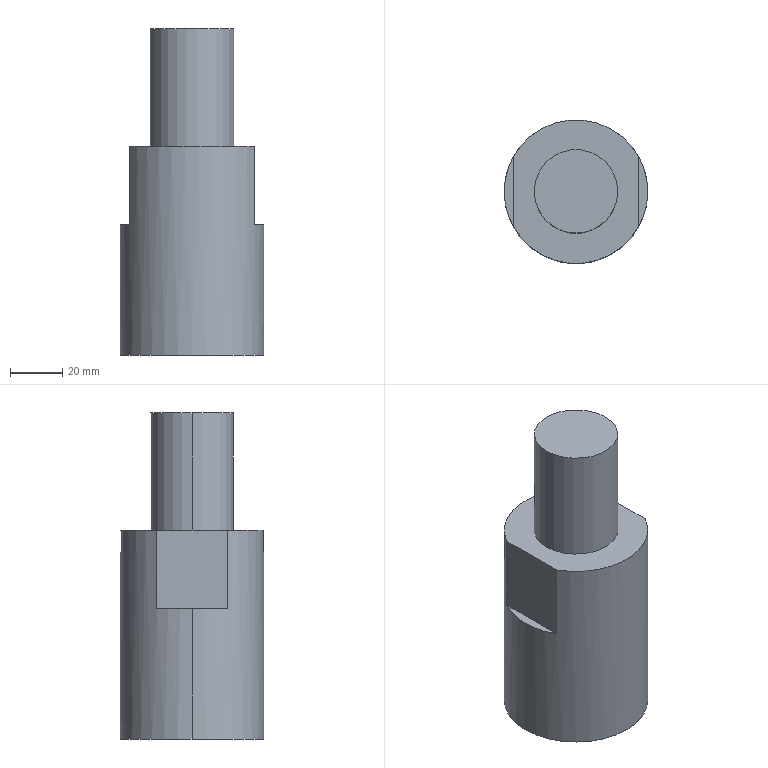Part | STEP file | 001-009-Riveting mechanism adapter joint | 1 solid | 15 faces | box 55 x 55 x 125 mm | volume 189803 mm3 | plane 7 | cylinder 6 | cone 2 | commonest cylinder face diameters 25 x2 32 x2 55 x2
STEP:
#1=CARTESIAN_POINT('',(0.,0.,0.));
#2=DIRECTION('',(0.,0.,1.));
#3=DIRECTION('',(1.,0.,0.));
#4=AXIS2_PLACEMENT_3D('',#1,#2,#3);
#5=CARTESIAN_POINT('',(-12.5,0.,64.));
#6=VERTEX_POINT('',#5);
#7=CARTESIAN_POINT('',(-12.5,0.,0.));
#8=VERTEX_POINT('',#7);
#9=CARTESIAN_POINT('',(-12.5,0.,0.));
#10=DIRECTION('',(0.,0.,-1.));
#11=VECTOR('',#10,1.);
#12=LINE('',#9,#11);
#13=CARTESIAN_POINT('',(0.,0.,0.));
#14=DIRECTION('',(0.,0.,-1.));
#15=DIRECTION('',(-1.,0.,0.));
#16=AXIS2_PLACEMENT_3D('',#13,#14,#15);
#17=CYLINDRICAL_SURFACE('',#16,12.5);
#18=CARTESIAN_POINT('',(6.283,0.));
#19=DIRECTION('',(0.,1.));
#20=VECTOR('',#19,1.);
#21=LINE('',#18,#20);
#22=(GEOMETRIC_REPRESENTATION_CONTEXT(2)PARAMETRIC_REPRESENTATION_CONTEXT()REPRESENTATION_CONTEXT('',''));
#23=DEFINITIONAL_REPRESENTATION('',(#21),#22);
#24=PCURVE('',#17,#23);
#25=CARTESIAN_POINT('',(0.,0.,0.));
#26=DIRECTION('',(0.,0.,-1.));
#27=DIRECTION('',(-1.,0.,0.));
#28=AXIS2_PLACEMENT_3D('',#25,#26,#27);
#29=CYLINDRICAL_SURFACE('',#28,12.5);
#30=CARTESIAN_POINT('',(0.,0.));
#31=DIRECTION('',(0.,1.));
#32=VECTOR('',#31,1.);
#33=LINE('',#30,#32);
#34=(GEOMETRIC_REPRESENTATION_CONTEXT(2)PARAMETRIC_REPRESENTATION_CONTEXT()REPRESENTATION_CONTEXT('',''));
#35=DEFINITIONAL_REPRESENTATION('',(#33),#34);
#36=PCURVE('',#29,#35);
#37=SURFACE_CURVE('',#12,(#24,#36),.PCURVE_S1.);
#38=EDGE_CURVE('',#6,#8,#37,.T.);
#39=ORIENTED_EDGE('',*,*,#38,.T.);
#40=CARTESIAN_POINT('',(12.5,0.,0.));
#41=VERTEX_POINT('',#40);
#42=CARTESIAN_POINT('',(0.,0.,0.));
#43=DIRECTION('',(0.,0.,-1.));
#44=DIRECTION('',(-1.,0.,0.));
#45=AXIS2_PLACEMENT_3D('',#42,#43,#44);
#46=CIRCLE('',#45,12.5);
#47=CARTESIAN_POINT('',(0.,0.));
#48=DIRECTION('',(1.,0.));
#49=VECTOR('',#48,1.);
#50=LINE('',#47,#49);
#51=(GEOMETRIC_REPRESENTATION_CONTEXT(2)PARAMETRIC_REPRESENTATION_CONTEXT()REPRESENTATION_CONTEXT('',''));
#52=DEFINITIONAL_REPRESENTATION('',(#50),#51);
#53=PCURVE('',#17,#52);
#54=CARTESIAN_POINT('',(0.,0.,0.));
#55=DIRECTION('',(0.,0.,1.));
#56=DIRECTION('',(1.,0.,0.));
#57=AXIS2_PLACEMENT_3D('',#54,#55,#56);
#58=PLANE('',#57);
#59=CARTESIAN_POINT('',(-12.5,0.));
#60=CARTESIAN_POINT('',(-12.5,21.651));
#61=CARTESIAN_POINT('',(6.25,10.825));
#62=CARTESIAN_POINT('',(25.,0.));
#63=CARTESIAN_POINT('',(6.25,-10.825));
#64=CARTESIAN_POINT('',(-12.5,-21.651));
#65=CARTESIAN_POINT('',(-12.5,0.));
#66=(BOUNDED_CURVE()B_SPLINE_CURVE(2,(#59,#60,#61,#62,#63,#64,#65),.UNSPECIFIED.,.T.,.F.)B_SPLINE_CURVE_WITH_KNOTS((1,2,2,2,2,1),(-2.094,0.,2.094,4.189,6.283,8.378),.UNSPECIFIED.)CURVE()GEOMETRIC_REPRESENTATION_ITEM()RATIONAL_B_SPLINE_CURVE((1.,0.5,1.,0.5,1.,0.5,1.))REPRESENTATION_ITEM(''));
#67=(GEOMETRIC_REPRESENTATION_CONTEXT(2)PARAMETRIC_REPRESENTATION_CONTEXT()REPRESENTATION_CONTEXT('',''));
#68=DEFINITIONAL_REPRESENTATION('',(#66),#67);
#69=PCURVE('',#58,#68);
#70=SURFACE_CURVE('',#46,(#53,#69),.PCURVE_S1.);
#71=EDGE_CURVE('',#41,#8,#70,.T.);
#72=ORIENTED_EDGE('',*,*,#71,.F.);
#73=CARTESIAN_POINT('',(12.5,0.,64.));
#74=VERTEX_POINT('',#73);
#75=CARTESIAN_POINT('',(12.5,0.,0.));
#76=DIRECTION('',(0.,0.,-1.));
#77=VECTOR('',#76,1.);
#78=LINE('',#75,#77);
#79=CARTESIAN_POINT('',(3.142,0.));
#80=DIRECTION('',(0.,1.));
#81=VECTOR('',#80,1.);
#82=LINE('',#79,#81);
#83=(GEOMETRIC_REPRESENTATION_CONTEXT(2)PARAMETRIC_REPRESENTATION_CONTEXT()REPRESENTATION_CONTEXT('',''));
#84=DEFINITIONAL_REPRESENTATION('',(#82),#83);
#85=PCURVE('',#17,#84);
#86=CARTESIAN_POINT('',(3.142,0.));
#87=DIRECTION('',(0.,1.));
#88=VECTOR('',#87,1.);
#89=LINE('',#86,#88);
#90=(GEOMETRIC_REPRESENTATION_CONTEXT(2)PARAMETRIC_REPRESENTATION_CONTEXT()REPRESENTATION_CONTEXT('',''));
#91=DEFINITIONAL_REPRESENTATION('',(#89),#90);
#92=PCURVE('',#29,#91);
#93=SURFACE_CURVE('',#78,(#85,#92),.PCURVE_S1.);
#94=EDGE_CURVE('',#74,#41,#93,.T.);
#95=ORIENTED_EDGE('',*,*,#94,.F.);
#96=CARTESIAN_POINT('',(0.,0.,64.));
#97=DIRECTION('',(0.,0.,-1.));
#98=DIRECTION('',(-1.,0.,0.));
#99=AXIS2_PLACEMENT_3D('',#96,#97,#98);
#100=CIRCLE('',#99,12.5);
#101=CARTESIAN_POINT('',(0.,-64.));
#102=DIRECTION('',(1.,0.));
#103=VECTOR('',#102,1.);
#104=LINE('',#101,#103);
#105=(GEOMETRIC_REPRESENTATION_CONTEXT(2)PARAMETRIC_REPRESENTATION_CONTEXT()REPRESENTATION_CONTEXT('',''));
#106=DEFINITIONAL_REPRESENTATION('',(#104),#105);
#107=PCURVE('',#17,#106);
#108=CARTESIAN_POINT('',(0.,0.,64.));
#109=DIRECTION('',(0.,0.,-1.));
#110=DIRECTION('',(-1.,0.,0.));
#111=AXIS2_PLACEMENT_3D('',#108,#109,#110);
#112=CONICAL_SURFACE('',#111,12.5,1.03);
#113=CARTESIAN_POINT('',(0.,0.));
#114=DIRECTION('',(1.,0.));
#115=VECTOR('',#114,1.);
#116=LINE('',#113,#115);
#117=(GEOMETRIC_REPRESENTATION_CONTEXT(2)PARAMETRIC_REPRESENTATION_CONTEXT()REPRESENTATION_CONTEXT('',''));
#118=DEFINITIONAL_REPRESENTATION('',(#116),#117);
#119=PCURVE('',#112,#118);
#120=SURFACE_CURVE('',#100,(#107,#119),.PCURVE_S1.);
#121=EDGE_CURVE('',#74,#6,#120,.T.);
#122=ORIENTED_EDGE('',*,*,#121,.T.);
#123=EDGE_LOOP('',(#39,#72,#95,#122));
#124=FACE_BOUND('',#123,.F.);
#125=ADVANCED_FACE('',(#124),#17,.F.);
#126=ORIENTED_EDGE('',*,*,#121,.F.);
#127=CARTESIAN_POINT('',(0.,0.,71.511));
#128=VERTEX_POINT('',#127);
#129=CARTESIAN_POINT('',(12.5,0.,64.));
#130=DIRECTION('',(0.8572,0.,-0.515));
#131=VECTOR('',#130,1.);
#132=LINE('',#129,#131);
#133=CARTESIAN_POINT('',(3.142,0.));
#134=DIRECTION('',(0.,1.));
#135=VECTOR('',#134,1.);
#136=LINE('',#133,#135);
#137=(GEOMETRIC_REPRESENTATION_CONTEXT(2)PARAMETRIC_REPRESENTATION_CONTEXT()REPRESENTATION_CONTEXT('',''));
#138=DEFINITIONAL_REPRESENTATION('',(#136),#137);
#139=PCURVE('',#112,#138);
#140=CARTESIAN_POINT('',(0.,0.,64.));
#141=DIRECTION('',(0.,0.,-1.));
#142=DIRECTION('',(-1.,0.,0.));
#143=AXIS2_PLACEMENT_3D('',#140,#141,#142);
#144=CONICAL_SURFACE('',#143,12.5,1.03);
#145=CARTESIAN_POINT('',(3.142,0.));
#146=DIRECTION('',(0.,1.));
#147=VECTOR('',#146,1.);
#148=LINE('',#145,#147);
#149=(GEOMETRIC_REPRESENTATION_CONTEXT(2)PARAMETRIC_REPRESENTATION_CONTEXT()REPRESENTATION_CONTEXT('',''));
#150=DEFINITIONAL_REPRESENTATION('',(#148),#149);
#151=PCURVE('',#144,#150);
#152=SURFACE_CURVE('',#132,(#139,#151),.PCURVE_S1.);
#153=EDGE_CURVE('',#128,#74,#152,.T.);
#154=ORIENTED_EDGE('',*,*,#153,.F.);
#155=CARTESIAN_POINT('',(-12.5,0.,64.));
#156=DIRECTION('',(-0.8572,0.,-0.515));
#157=VECTOR('',#156,1.);
#158=LINE('',#155,#157);
#159=CARTESIAN_POINT('',(6.283,0.));
#160=DIRECTION('',(0.,1.));
#161=VECTOR('',#160,1.);
#162=LINE('',#159,#161);
#163=(GEOMETRIC_REPRESENTATION_CONTEXT(2)PARAMETRIC_REPRESENTATION_CONTEXT()REPRESENTATION_CONTEXT('',''));
#164=DEFINITIONAL_REPRESENTATION('',(#162),#163);
#165=PCURVE('',#112,#164);
#166=CARTESIAN_POINT('',(0.,0.));
#167=DIRECTION('',(0.,1.));
#168=VECTOR('',#167,1.);
#169=LINE('',#166,#168);
#170=(GEOMETRIC_REPRESENTATION_CONTEXT(2)PARAMETRIC_REPRESENTATION_CONTEXT()REPRESENTATION_CONTEXT('',''));
#171=DEFINITIONAL_REPRESENTATION('',(#169),#170);
#172=PCURVE('',#144,#171);
#173=SURFACE_CURVE('',#158,(#165,#172),.PCURVE_S1.);
#174=EDGE_CURVE('',#128,#6,#173,.T.);
#175=ORIENTED_EDGE('',*,*,#174,.T.);
#176=EDGE_LOOP('',(#126,#154,#175));
#177=FACE_BOUND('',#176,.F.);
#178=ADVANCED_FACE('',(#177),#112,.F.);
#179=CARTESIAN_POINT('',(16.,0.,125.));
#180=VERTEX_POINT('',#179);
#181=CARTESIAN_POINT('',(-16.,0.,125.));
#182=VERTEX_POINT('',#181);
#183=CARTESIAN_POINT('',(0.,0.,125.));
#184=DIRECTION('',(0.,0.,1.));
#185=DIRECTION('',(1.,0.,0.));
#186=AXIS2_PLACEMENT_3D('',#183,#184,#185);
#187=CIRCLE('',#186,16.);
#188=CARTESIAN_POINT('',(0.,0.,125.));
#189=DIRECTION('',(0.,0.,-1.));
#190=DIRECTION('',(-1.,0.,0.));
#191=AXIS2_PLACEMENT_3D('',#188,#189,#190);
#192=CYLINDRICAL_SURFACE('',#191,16.);
#193=CARTESIAN_POINT('',(3.142,0.));
#194=DIRECTION('',(-1.,0.));
#195=VECTOR('',#194,1.);
#196=LINE('',#193,#195);
#197=(GEOMETRIC_REPRESENTATION_CONTEXT(2)PARAMETRIC_REPRESENTATION_CONTEXT()REPRESENTATION_CONTEXT('',''));
#198=DEFINITIONAL_REPRESENTATION('',(#196),#197);
#199=PCURVE('',#192,#198);
#200=CARTESIAN_POINT('',(0.,0.,125.));
#201=DIRECTION('',(0.,0.,1.));
#202=DIRECTION('',(1.,0.,0.));
#203=AXIS2_PLACEMENT_3D('',#200,#201,#202);
#204=PLANE('',#203);
#205=CARTESIAN_POINT('',(0.,0.));
#206=DIRECTION('',(1.,0.));
#207=AXIS2_PLACEMENT_2D('',#205,#206);
#208=CIRCLE('',#207,16.);
#209=(GEOMETRIC_REPRESENTATION_CONTEXT(2)PARAMETRIC_REPRESENTATION_CONTEXT()REPRESENTATION_CONTEXT('',''));
#210=DEFINITIONAL_REPRESENTATION('',(#208),#209);
#211=PCURVE('',#204,#210);
#212=SURFACE_CURVE('',#187,(#199,#211),.PCURVE_S1.);
#213=EDGE_CURVE('',#180,#182,#212,.T.);
#214=ORIENTED_EDGE('',*,*,#213,.F.);
#215=CARTESIAN_POINT('',(16.,0.,80.));
#216=VERTEX_POINT('',#215);
#217=CARTESIAN_POINT('',(16.,0.,125.));
#218=DIRECTION('',(0.,0.,-1.));
#219=VECTOR('',#218,1.);
#220=LINE('',#217,#219);
#221=CARTESIAN_POINT('',(3.142,0.));
#222=DIRECTION('',(0.,1.));
#223=VECTOR('',#222,1.);
#224=LINE('',#221,#223);
#225=(GEOMETRIC_REPRESENTATION_CONTEXT(2)PARAMETRIC_REPRESENTATION_CONTEXT()REPRESENTATION_CONTEXT('',''));
#226=DEFINITIONAL_REPRESENTATION('',(#224),#225);
#227=PCURVE('',#192,#226);
#228=CARTESIAN_POINT('',(0.,0.,125.));
#229=DIRECTION('',(0.,0.,-1.));
#230=DIRECTION('',(-1.,0.,0.));
#231=AXIS2_PLACEMENT_3D('',#228,#229,#230);
#232=CYLINDRICAL_SURFACE('',#231,16.);
#233=CARTESIAN_POINT('',(3.142,0.));
#234=DIRECTION('',(0.,1.));
#235=VECTOR('',#234,1.);
#236=LINE('',#233,#235);
#237=(GEOMETRIC_REPRESENTATION_CONTEXT(2)PARAMETRIC_REPRESENTATION_CONTEXT()REPRESENTATION_CONTEXT('',''));
#238=DEFINITIONAL_REPRESENTATION('',(#236),#237);
#239=PCURVE('',#232,#238);
#240=SURFACE_CURVE('',#220,(#227,#239),.PCURVE_S1.);
#241=EDGE_CURVE('',#180,#216,#240,.T.);
#242=ORIENTED_EDGE('',*,*,#241,.T.);
#243=CARTESIAN_POINT('',(-16.,0.,80.));
#244=VERTEX_POINT('',#243);
#245=CARTESIAN_POINT('',(0.,0.,80.));
#246=DIRECTION('',(0.,0.,1.));
#247=DIRECTION('',(1.,0.,0.));
#248=AXIS2_PLACEMENT_3D('',#245,#246,#247);
#249=CIRCLE('',#248,16.);
#250=CARTESIAN_POINT('',(3.142,45.));
#251=DIRECTION('',(-1.,0.));
#252=VECTOR('',#251,1.);
#253=LINE('',#250,#252);
#254=(GEOMETRIC_REPRESENTATION_CONTEXT(2)PARAMETRIC_REPRESENTATION_CONTEXT()REPRESENTATION_CONTEXT('',''));
#255=DEFINITIONAL_REPRESENTATION('',(#253),#254);
#256=PCURVE('',#192,#255);
#257=CARTESIAN_POINT('',(0.,0.,80.));
#258=DIRECTION('',(0.,0.,1.));
#259=DIRECTION('',(1.,0.,0.));
#260=AXIS2_PLACEMENT_3D('',#257,#258,#259);
#261=PLANE('',#260);
#262=CARTESIAN_POINT('',(0.,0.));
#263=DIRECTION('',(1.,0.));
#264=AXIS2_PLACEMENT_2D('',#262,#263);
#265=CIRCLE('',#264,16.);
#266=(GEOMETRIC_REPRESENTATION_CONTEXT(2)PARAMETRIC_REPRESENTATION_CONTEXT()REPRESENTATION_CONTEXT('',''));
#267=DEFINITIONAL_REPRESENTATION('',(#265),#266);
#268=PCURVE('',#261,#267);
#269=SURFACE_CURVE('',#249,(#256,#268),.PCURVE_S1.);
#270=EDGE_CURVE('',#216,#244,#269,.T.);
#271=ORIENTED_EDGE('',*,*,#270,.T.);
#272=CARTESIAN_POINT('',(-16.,0.,125.));
#273=DIRECTION('',(0.,0.,-1.));
#274=VECTOR('',#273,1.);
#275=LINE('',#272,#274);
#276=CARTESIAN_POINT('',(0.,0.));
#277=DIRECTION('',(0.,1.));
#278=VECTOR('',#277,1.);
#279=LINE('',#276,#278);
#280=(GEOMETRIC_REPRESENTATION_CONTEXT(2)PARAMETRIC_REPRESENTATION_CONTEXT()REPRESENTATION_CONTEXT('',''));
#281=DEFINITIONAL_REPRESENTATION('',(#279),#280);
#282=PCURVE('',#192,#281);
#283=CARTESIAN_POINT('',(6.283,0.));
#284=DIRECTION('',(0.,1.));
#285=VECTOR('',#284,1.);
#286=LINE('',#283,#285);
#287=(GEOMETRIC_REPRESENTATION_CONTEXT(2)PARAMETRIC_REPRESENTATION_CONTEXT()REPRESENTATION_CONTEXT('',''));
#288=DEFINITIONAL_REPRESENTATION('',(#286),#287);
#289=PCURVE('',#232,#288);
#290=SURFACE_CURVE('',#275,(#282,#289),.PCURVE_S1.);
#291=EDGE_CURVE('',#182,#244,#290,.T.);
#292=ORIENTED_EDGE('',*,*,#291,.F.);
#293=EDGE_LOOP('',(#214,#242,#271,#292));
#294=FACE_BOUND('',#293,.T.);
#295=ADVANCED_FACE('',(#294),#192,.T.);
#296=CARTESIAN_POINT('',(27.5,0.,50.));
#297=VERTEX_POINT('',#296);
#298=CARTESIAN_POINT('',(24.,13.426,50.));
#299=VERTEX_POINT('',#298);
#300=CARTESIAN_POINT('',(0.,0.,50.));
#301=DIRECTION('',(0.,0.,1.));
#302=DIRECTION('',(1.,0.,0.));
#303=AXIS2_PLACEMENT_3D('',#300,#301,#302);
#304=CIRCLE('',#303,27.5);
#305=CARTESIAN_POINT('',(0.,0.,80.));
#306=DIRECTION('',(0.,0.,-1.));
#307=DIRECTION('',(-1.,0.,0.));
#308=AXIS2_PLACEMENT_3D('',#305,#306,#307);
#309=CYLINDRICAL_SURFACE('',#308,27.5);
#310=CARTESIAN_POINT('',(3.142,30.));
#311=DIRECTION('',(-1.,0.));
#312=VECTOR('',#311,1.);
#313=LINE('',#310,#312);
#314=(GEOMETRIC_REPRESENTATION_CONTEXT(2)PARAMETRIC_REPRESENTATION_CONTEXT()REPRESENTATION_CONTEXT('',''));
#315=DEFINITIONAL_REPRESENTATION('',(#313),#314);
#316=PCURVE('',#309,#315);
#317=CARTESIAN_POINT('',(0.,0.,50.));
#318=DIRECTION('',(0.,0.,1.));
#319=DIRECTION('',(1.,0.,0.));
#320=AXIS2_PLACEMENT_3D('',#317,#318,#319);
#321=PLANE('',#320);
#322=CARTESIAN_POINT('',(0.,0.));
#323=DIRECTION('',(1.,0.));
#324=AXIS2_PLACEMENT_2D('',#322,#323);
#325=CIRCLE('',#324,27.5);
#326=(GEOMETRIC_REPRESENTATION_CONTEXT(2)PARAMETRIC_REPRESENTATION_CONTEXT()REPRESENTATION_CONTEXT('',''));
#327=DEFINITIONAL_REPRESENTATION('',(#325),#326);
#328=PCURVE('',#321,#327);
#329=SURFACE_CURVE('',#304,(#316,#328),.PCURVE_S1.);
#330=EDGE_CURVE('',#297,#299,#329,.T.);
#331=ORIENTED_EDGE('',*,*,#330,.F.);
#332=CARTESIAN_POINT('',(27.5,0.,0.));
#333=VERTEX_POINT('',#332);
#334=CARTESIAN_POINT('',(27.5,0.,80.));
#335=DIRECTION('',(0.,0.,-1.));
#336=VECTOR('',#335,1.);
#337=LINE('',#334,#336);
#338=CARTESIAN_POINT('',(3.142,0.));
#339=DIRECTION('',(0.,1.));
#340=VECTOR('',#339,1.);
#341=LINE('',#338,#340);
#342=(GEOMETRIC_REPRESENTATION_CONTEXT(2)PARAMETRIC_REPRESENTATION_CONTEXT()REPRESENTATION_CONTEXT('',''));
#343=DEFINITIONAL_REPRESENTATION('',(#341),#342);
#344=PCURVE('',#309,#343);
#345=CARTESIAN_POINT('',(0.,0.,80.));
#346=DIRECTION('',(0.,0.,-1.));
#347=DIRECTION('',(-1.,0.,0.));
#348=AXIS2_PLACEMENT_3D('',#345,#346,#347);
#349=CYLINDRICAL_SURFACE('',#348,27.5);
#350=CARTESIAN_POINT('',(3.142,0.));
#351=DIRECTION('',(0.,1.));
#352=VECTOR('',#351,1.);
#353=LINE('',#350,#352);
#354=(GEOMETRIC_REPRESENTATION_CONTEXT(2)PARAMETRIC_REPRESENTATION_CONTEXT()REPRESENTATION_CONTEXT('',''));
#355=DEFINITIONAL_REPRESENTATION('',(#353),#354);
#356=PCURVE('',#349,#355);
#357=SURFACE_CURVE('',#337,(#344,#356),.PCURVE_S1.);
#358=EDGE_CURVE('',#297,#333,#357,.T.);
#359=ORIENTED_EDGE('',*,*,#358,.T.);
#360=CARTESIAN_POINT('',(-27.5,0.,0.));
#361=VERTEX_POINT('',#360);
#362=CARTESIAN_POINT('',(0.,0.,0.));
#363=DIRECTION('',(0.,0.,1.));
#364=DIRECTION('',(1.,0.,0.));
#365=AXIS2_PLACEMENT_3D('',#362,#363,#364);
#366=CIRCLE('',#365,27.5);
#367=CARTESIAN_POINT('',(3.142,80.));
#368=DIRECTION('',(-1.,0.));
#369=VECTOR('',#368,1.);
#370=LINE('',#367,#369);
#371=(GEOMETRIC_REPRESENTATION_CONTEXT(2)PARAMETRIC_REPRESENTATION_CONTEXT()REPRESENTATION_CONTEXT('',''));
#372=DEFINITIONAL_REPRESENTATION('',(#370),#371);
#373=PCURVE('',#309,#372);
#374=CARTESIAN_POINT('',(0.,0.));
#375=DIRECTION('',(1.,0.));
#376=AXIS2_PLACEMENT_2D('',#374,#375);
#377=CIRCLE('',#376,27.5);
#378=(GEOMETRIC_REPRESENTATION_CONTEXT(2)PARAMETRIC_REPRESENTATION_CONTEXT()REPRESENTATION_CONTEXT('',''));
#379=DEFINITIONAL_REPRESENTATION('',(#377),#378);
#380=PCURVE('',#58,#379);
#381=SURFACE_CURVE('',#366,(#373,#380),.PCURVE_S1.);
#382=EDGE_CURVE('',#333,#361,#381,.T.);
#383=ORIENTED_EDGE('',*,*,#382,.T.);
#384=CARTESIAN_POINT('',(-27.5,0.,50.));
#385=VERTEX_POINT('',#384);
#386=CARTESIAN_POINT('',(-27.5,0.,80.));
#387=DIRECTION('',(0.,0.,-1.));
#388=VECTOR('',#387,1.);
#389=LINE('',#386,#388);
#390=CARTESIAN_POINT('',(0.,0.));
#391=DIRECTION('',(0.,1.));
#392=VECTOR('',#391,1.);
#393=LINE('',#390,#392);
#394=(GEOMETRIC_REPRESENTATION_CONTEXT(2)PARAMETRIC_REPRESENTATION_CONTEXT()REPRESENTATION_CONTEXT('',''));
#395=DEFINITIONAL_REPRESENTATION('',(#393),#394);
#396=PCURVE('',#309,#395);
#397=CARTESIAN_POINT('',(6.283,0.));
#398=DIRECTION('',(0.,1.));
#399=VECTOR('',#398,1.);
#400=LINE('',#397,#399);
#401=(GEOMETRIC_REPRESENTATION_CONTEXT(2)PARAMETRIC_REPRESENTATION_CONTEXT()REPRESENTATION_CONTEXT('',''));
#402=DEFINITIONAL_REPRESENTATION('',(#400),#401);
#403=PCURVE('',#349,#402);
#404=SURFACE_CURVE('',#389,(#396,#403),.PCURVE_S1.);
#405=EDGE_CURVE('',#385,#361,#404,.T.);
#406=ORIENTED_EDGE('',*,*,#405,.F.);
#407=CARTESIAN_POINT('',(-24.,13.426,50.));
#408=VERTEX_POINT('',#407);
#409=CARTESIAN_POINT('',(0.,0.,50.));
#410=DIRECTION('',(0.,0.,1.));
#411=DIRECTION('',(1.,0.,0.));
#412=AXIS2_PLACEMENT_3D('',#409,#410,#411);
#413=CIRCLE('',#412,27.5);
#414=CARTESIAN_POINT('',(3.142,30.));
#415=DIRECTION('',(-1.,0.));
#416=VECTOR('',#415,1.);
#417=LINE('',#414,#416);
#418=(GEOMETRIC_REPRESENTATION_CONTEXT(2)PARAMETRIC_REPRESENTATION_CONTEXT()REPRESENTATION_CONTEXT('',''));
#419=DEFINITIONAL_REPRESENTATION('',(#417),#418);
#420=PCURVE('',#309,#419);
#421=CARTESIAN_POINT('',(0.,0.,50.));
#422=DIRECTION('',(0.,0.,1.));
#423=DIRECTION('',(1.,0.,0.));
#424=AXIS2_PLACEMENT_3D('',#421,#422,#423);
#425=PLANE('',#424);
#426=CARTESIAN_POINT('',(0.,0.));
#427=DIRECTION('',(1.,0.));
#428=AXIS2_PLACEMENT_2D('',#426,#427);
#429=CIRCLE('',#428,27.5);
#430=(GEOMETRIC_REPRESENTATION_CONTEXT(2)PARAMETRIC_REPRESENTATION_CONTEXT()REPRESENTATION_CONTEXT('',''));
#431=DEFINITIONAL_REPRESENTATION('',(#429),#430);
#432=PCURVE('',#425,#431);
#433=SURFACE_CURVE('',#413,(#420,#432),.PCURVE_S1.);
#434=EDGE_CURVE('',#408,#385,#433,.T.);
#435=ORIENTED_EDGE('',*,*,#434,.F.);
#436=CARTESIAN_POINT('',(-24.,13.426,80.));
#437=VERTEX_POINT('',#436);
#438=CARTESIAN_POINT('',(-24.,13.426,80.));
#439=DIRECTION('',(0.,0.,-1.));
#440=VECTOR('',#439,1.);
#441=LINE('',#438,#440);
#442=CARTESIAN_POINT('',(0.51,0.));
#443=DIRECTION('',(0.,1.));
#444=VECTOR('',#443,1.);
#445=LINE('',#442,#444);
#446=(GEOMETRIC_REPRESENTATION_CONTEXT(2)PARAMETRIC_REPRESENTATION_CONTEXT()REPRESENTATION_CONTEXT('',''));
#447=DEFINITIONAL_REPRESENTATION('',(#445),#446);
#448=PCURVE('',#309,#447);
#449=CARTESIAN_POINT('',(-24.,-32.5,50.));
#450=DIRECTION('',(-1.,0.,0.));
#451=DIRECTION('',(0.,-1.,0.));
#452=AXIS2_PLACEMENT_3D('',#449,#450,#451);
#453=PLANE('',#452);
#454=CARTESIAN_POINT('',(-45.926,30.));
#455=DIRECTION('',(0.,-1.));
#456=VECTOR('',#455,1.);
#457=LINE('',#454,#456);
#458=(GEOMETRIC_REPRESENTATION_CONTEXT(2)PARAMETRIC_REPRESENTATION_CONTEXT()REPRESENTATION_CONTEXT('',''));
#459=DEFINITIONAL_REPRESENTATION('',(#457),#458);
#460=PCURVE('',#453,#459);
#461=SURFACE_CURVE('',#441,(#448,#460),.PCURVE_S1.);
#462=EDGE_CURVE('',#437,#408,#461,.T.);
#463=ORIENTED_EDGE('',*,*,#462,.F.);
#464=CARTESIAN_POINT('',(24.,13.426,80.));
#465=VERTEX_POINT('',#464);
#466=CARTESIAN_POINT('',(0.,0.,80.));
#467=DIRECTION('',(0.,0.,1.));
#468=DIRECTION('',(1.,0.,0.));
#469=AXIS2_PLACEMENT_3D('',#466,#467,#468);
#470=CIRCLE('',#469,27.5);
#471=CARTESIAN_POINT('',(3.142,0.));
#472=DIRECTION('',(-1.,0.));
#473=VECTOR('',#472,1.);
#474=LINE('',#471,#473);
#475=(GEOMETRIC_REPRESENTATION_CONTEXT(2)PARAMETRIC_REPRESENTATION_CONTEXT()REPRESENTATION_CONTEXT('',''));
#476=DEFINITIONAL_REPRESENTATION('',(#474),#475);
#477=PCURVE('',#309,#476);
#478=CARTESIAN_POINT('',(0.,0.));
#479=DIRECTION('',(1.,0.));
#480=AXIS2_PLACEMENT_2D('',#478,#479);
#481=CIRCLE('',#480,27.5);
#482=(GEOMETRIC_REPRESENTATION_CONTEXT(2)PARAMETRIC_REPRESENTATION_CONTEXT()REPRESENTATION_CONTEXT('',''));
#483=DEFINITIONAL_REPRESENTATION('',(#481),#482);
#484=PCURVE('',#261,#483);
#485=SURFACE_CURVE('',#470,(#477,#484),.PCURVE_S1.);
#486=EDGE_CURVE('',#465,#437,#485,.T.);
#487=ORIENTED_EDGE('',*,*,#486,.F.);
#488=CARTESIAN_POINT('',(24.,13.426,80.));
#489=DIRECTION('',(0.,0.,1.));
#490=VECTOR('',#489,1.);
#491=LINE('',#488,#490);
#492=CARTESIAN_POINT('',(2.632,0.));
#493=DIRECTION('',(0.,-1.));
#494=VECTOR('',#493,1.);
#495=LINE('',#492,#494);
#496=(GEOMETRIC_REPRESENTATION_CONTEXT(2)PARAMETRIC_REPRESENTATION_CONTEXT()REPRESENTATION_CONTEXT('',''));
#497=DEFINITIONAL_REPRESENTATION('',(#495),#496);
#498=PCURVE('',#309,#497);
#499=CARTESIAN_POINT('',(24.,-32.5,50.));
#500=DIRECTION('',(1.,0.,0.));
#501=DIRECTION('',(0.,1.,0.));
#502=AXIS2_PLACEMENT_3D('',#499,#500,#501);
#503=PLANE('',#502);
#504=CARTESIAN_POINT('',(45.926,30.));
#505=DIRECTION('',(0.,1.));
#506=VECTOR('',#505,1.);
#507=LINE('',#504,#506);
#508=(GEOMETRIC_REPRESENTATION_CONTEXT(2)PARAMETRIC_REPRESENTATION_CONTEXT()REPRESENTATION_CONTEXT('',''));
#509=DEFINITIONAL_REPRESENTATION('',(#507),#508);
#510=PCURVE('',#503,#509);
#511=SURFACE_CURVE('',#491,(#498,#510),.PCURVE_S1.);
#512=EDGE_CURVE('',#299,#465,#511,.T.);
#513=ORIENTED_EDGE('',*,*,#512,.F.);
#514=EDGE_LOOP('',(#331,#359,#383,#406,#435,#463,#487,#513));
#515=FACE_BOUND('',#514,.T.);
#516=ADVANCED_FACE('',(#515),#309,.T.);
#517=ORIENTED_EDGE('',*,*,#358,.F.);
#518=CARTESIAN_POINT('',(24.,-13.426,50.));
#519=VERTEX_POINT('',#518);
#520=CARTESIAN_POINT('',(0.,0.,50.));
#521=DIRECTION('',(0.,0.,1.));
#522=DIRECTION('',(1.,0.,0.));
#523=AXIS2_PLACEMENT_3D('',#520,#521,#522);
#524=CIRCLE('',#523,27.5);
#525=CARTESIAN_POINT('',(9.425,30.));
#526=DIRECTION('',(-1.,0.));
#527=VECTOR('',#526,1.);
#528=LINE('',#525,#527);
#529=(GEOMETRIC_REPRESENTATION_CONTEXT(2)PARAMETRIC_REPRESENTATION_CONTEXT()REPRESENTATION_CONTEXT('',''));
#530=DEFINITIONAL_REPRESENTATION('',(#528),#529);
#531=PCURVE('',#349,#530);
#532=CARTESIAN_POINT('',(0.,0.));
#533=DIRECTION('',(1.,0.));
#534=AXIS2_PLACEMENT_2D('',#532,#533);
#535=CIRCLE('',#534,27.5);
#536=(GEOMETRIC_REPRESENTATION_CONTEXT(2)PARAMETRIC_REPRESENTATION_CONTEXT()REPRESENTATION_CONTEXT('',''));
#537=DEFINITIONAL_REPRESENTATION('',(#535),#536);
#538=PCURVE('',#321,#537);
#539=SURFACE_CURVE('',#524,(#531,#538),.PCURVE_S1.);
#540=EDGE_CURVE('',#519,#297,#539,.T.);
#541=ORIENTED_EDGE('',*,*,#540,.F.);
#542=CARTESIAN_POINT('',(24.,-13.426,80.));
#543=VERTEX_POINT('',#542);
#544=CARTESIAN_POINT('',(24.,-13.426,80.));
#545=DIRECTION('',(0.,0.,-1.));
#546=VECTOR('',#545,1.);
#547=LINE('',#544,#546);
#548=CARTESIAN_POINT('',(3.652,0.));
#549=DIRECTION('',(0.,1.));
#550=VECTOR('',#549,1.);
#551=LINE('',#548,#550);
#552=(GEOMETRIC_REPRESENTATION_CONTEXT(2)PARAMETRIC_REPRESENTATION_CONTEXT()REPRESENTATION_CONTEXT('',''));
#553=DEFINITIONAL_REPRESENTATION('',(#551),#552);
#554=PCURVE('',#349,#553);
#555=CARTESIAN_POINT('',(19.074,30.));
#556=DIRECTION('',(0.,-1.));
#557=VECTOR('',#556,1.);
#558=LINE('',#555,#557);
#559=(GEOMETRIC_REPRESENTATION_CONTEXT(2)PARAMETRIC_REPRESENTATION_CONTEXT()REPRESENTATION_CONTEXT('',''));
#560=DEFINITIONAL_REPRESENTATION('',(#558),#559);
#561=PCURVE('',#503,#560);
#562=SURFACE_CURVE('',#547,(#554,#561),.PCURVE_S1.);
#563=EDGE_CURVE('',#543,#519,#562,.T.);
#564=ORIENTED_EDGE('',*,*,#563,.F.);
#565=CARTESIAN_POINT('',(-24.,-13.426,80.));
#566=VERTEX_POINT('',#565);
#567=CARTESIAN_POINT('',(0.,0.,80.));
#568=DIRECTION('',(0.,0.,1.));
#569=DIRECTION('',(1.,0.,0.));
#570=AXIS2_PLACEMENT_3D('',#567,#568,#569);
#571=CIRCLE('',#570,27.5);
#572=CARTESIAN_POINT('',(9.425,0.));
#573=DIRECTION('',(-1.,0.));
#574=VECTOR('',#573,1.);
#575=LINE('',#572,#574);
#576=(GEOMETRIC_REPRESENTATION_CONTEXT(2)PARAMETRIC_REPRESENTATION_CONTEXT()REPRESENTATION_CONTEXT('',''));
#577=DEFINITIONAL_REPRESENTATION('',(#575),#576);
#578=PCURVE('',#349,#577);
#579=CARTESIAN_POINT('',(0.,0.));
#580=DIRECTION('',(1.,0.));
#581=AXIS2_PLACEMENT_2D('',#579,#580);
#582=CIRCLE('',#581,27.5);
#583=(GEOMETRIC_REPRESENTATION_CONTEXT(2)PARAMETRIC_REPRESENTATION_CONTEXT()REPRESENTATION_CONTEXT('',''));
#584=DEFINITIONAL_REPRESENTATION('',(#582),#583);
#585=PCURVE('',#261,#584);
#586=SURFACE_CURVE('',#571,(#578,#585),.PCURVE_S1.);
#587=EDGE_CURVE('',#566,#543,#586,.T.);
#588=ORIENTED_EDGE('',*,*,#587,.F.);
#589=CARTESIAN_POINT('',(-24.,-13.426,50.));
#590=VERTEX_POINT('',#589);
#591=CARTESIAN_POINT('',(-24.,-13.426,80.));
#592=DIRECTION('',(0.,0.,1.));
#593=VECTOR('',#592,1.);
#594=LINE('',#591,#593);
#595=CARTESIAN_POINT('',(5.773,0.));
#596=DIRECTION('',(0.,-1.));
#597=VECTOR('',#596,1.);
#598=LINE('',#595,#597);
#599=(GEOMETRIC_REPRESENTATION_CONTEXT(2)PARAMETRIC_REPRESENTATION_CONTEXT()REPRESENTATION_CONTEXT('',''));
#600=DEFINITIONAL_REPRESENTATION('',(#598),#599);
#601=PCURVE('',#349,#600);
#602=CARTESIAN_POINT('',(-19.074,30.));
#603=DIRECTION('',(0.,1.));
#604=VECTOR('',#603,1.);
#605=LINE('',#602,#604);
#606=(GEOMETRIC_REPRESENTATION_CONTEXT(2)PARAMETRIC_REPRESENTATION_CONTEXT()REPRESENTATION_CONTEXT('',''));
#607=DEFINITIONAL_REPRESENTATION('',(#605),#606);
#608=PCURVE('',#453,#607);
#609=SURFACE_CURVE('',#594,(#601,#608),.PCURVE_S1.);
#610=EDGE_CURVE('',#590,#566,#609,.T.);
#611=ORIENTED_EDGE('',*,*,#610,.F.);
#612=CARTESIAN_POINT('',(0.,0.,50.));
#613=DIRECTION('',(0.,0.,1.));
#614=DIRECTION('',(1.,0.,0.));
#615=AXIS2_PLACEMENT_3D('',#612,#613,#614);
#616=CIRCLE('',#615,27.5);
#617=CARTESIAN_POINT('',(9.425,30.));
#618=DIRECTION('',(-1.,0.));
#619=VECTOR('',#618,1.);
#620=LINE('',#617,#619);
#621=(GEOMETRIC_REPRESENTATION_CONTEXT(2)PARAMETRIC_REPRESENTATION_CONTEXT()REPRESENTATION_CONTEXT('',''));
#622=DEFINITIONAL_REPRESENTATION('',(#620),#621);
#623=PCURVE('',#349,#622);
#624=CARTESIAN_POINT('',(0.,0.));
#625=DIRECTION('',(1.,0.));
#626=AXIS2_PLACEMENT_2D('',#624,#625);
#627=CIRCLE('',#626,27.5);
#628=(GEOMETRIC_REPRESENTATION_CONTEXT(2)PARAMETRIC_REPRESENTATION_CONTEXT()REPRESENTATION_CONTEXT('',''));
#629=DEFINITIONAL_REPRESENTATION('',(#627),#628);
#630=PCURVE('',#425,#629);
#631=SURFACE_CURVE('',#616,(#623,#630),.PCURVE_S1.);
#632=EDGE_CURVE('',#385,#590,#631,.T.);
#633=ORIENTED_EDGE('',*,*,#632,.F.);
#634=ORIENTED_EDGE('',*,*,#405,.T.);
#635=CARTESIAN_POINT('',(0.,0.,0.));
#636=DIRECTION('',(0.,0.,1.));
#637=DIRECTION('',(1.,0.,0.));
#638=AXIS2_PLACEMENT_3D('',#635,#636,#637);
#639=CIRCLE('',#638,27.5);
#640=CARTESIAN_POINT('',(9.425,80.));
#641=DIRECTION('',(-1.,0.));
#642=VECTOR('',#641,1.);
#643=LINE('',#640,#642);
#644=(GEOMETRIC_REPRESENTATION_CONTEXT(2)PARAMETRIC_REPRESENTATION_CONTEXT()REPRESENTATION_CONTEXT('',''));
#645=DEFINITIONAL_REPRESENTATION('',(#643),#644);
#646=PCURVE('',#349,#645);
#647=CARTESIAN_POINT('',(0.,0.));
#648=DIRECTION('',(1.,0.));
#649=AXIS2_PLACEMENT_2D('',#647,#648);
#650=CIRCLE('',#649,27.5);
#651=(GEOMETRIC_REPRESENTATION_CONTEXT(2)PARAMETRIC_REPRESENTATION_CONTEXT()REPRESENTATION_CONTEXT('',''));
#652=DEFINITIONAL_REPRESENTATION('',(#650),#651);
#653=PCURVE('',#58,#652);
#654=SURFACE_CURVE('',#639,(#646,#653),.PCURVE_S1.);
#655=EDGE_CURVE('',#361,#333,#654,.T.);
#656=ORIENTED_EDGE('',*,*,#655,.T.);
#657=EDGE_LOOP('',(#517,#541,#564,#588,#611,#633,#634,#656));
#658=FACE_BOUND('',#657,.T.);
#659=ADVANCED_FACE('',(#658),#349,.T.);
#660=CARTESIAN_POINT('',(0.,0.,80.));
#661=DIRECTION('',(0.,0.,1.));
#662=DIRECTION('',(1.,0.,0.));
#663=AXIS2_PLACEMENT_3D('',#660,#661,#662);
#664=CIRCLE('',#663,16.);
#665=CARTESIAN_POINT('',(0.,0.));
#666=DIRECTION('',(1.,0.));
#667=AXIS2_PLACEMENT_2D('',#665,#666);
#668=CIRCLE('',#667,16.);
#669=(GEOMETRIC_REPRESENTATION_CONTEXT(2)PARAMETRIC_REPRESENTATION_CONTEXT()REPRESENTATION_CONTEXT('',''));
#670=DEFINITIONAL_REPRESENTATION('',(#668),#669);
#671=PCURVE('',#261,#670);
#672=CARTESIAN_POINT('',(9.425,45.));
#673=DIRECTION('',(-1.,0.));
#674=VECTOR('',#673,1.);
#675=LINE('',#672,#674);
#676=(GEOMETRIC_REPRESENTATION_CONTEXT(2)PARAMETRIC_REPRESENTATION_CONTEXT()REPRESENTATION_CONTEXT('',''));
#677=DEFINITIONAL_REPRESENTATION('',(#675),#676);
#678=PCURVE('',#232,#677);
#679=SURFACE_CURVE('',#664,(#671,#678),.PCURVE_S1.);
#680=EDGE_CURVE('',#244,#216,#679,.T.);
#681=ORIENTED_EDGE('',*,*,#680,.F.);
#682=ORIENTED_EDGE('',*,*,#270,.F.);
#683=EDGE_LOOP('',(#681,#682));
#684=FACE_BOUND('',#683,.T.);
#685=ORIENTED_EDGE('',*,*,#587,.T.);
#686=CARTESIAN_POINT('',(24.,0.,80.));
#687=DIRECTION('',(0.,1.,0.));
#688=VECTOR('',#687,1.);
#689=LINE('',#686,#688);
#690=CARTESIAN_POINT('',(24.,0.));
#691=DIRECTION('',(0.,1.));
#692=VECTOR('',#691,1.);
#693=LINE('',#690,#692);
#694=(GEOMETRIC_REPRESENTATION_CONTEXT(2)PARAMETRIC_REPRESENTATION_CONTEXT()REPRESENTATION_CONTEXT('',''));
#695=DEFINITIONAL_REPRESENTATION('',(#693),#694);
#696=PCURVE('',#261,#695);
#697=CARTESIAN_POINT('',(32.5,30.));
#698=DIRECTION('',(1.,0.));
#699=VECTOR('',#698,1.);
#700=LINE('',#697,#699);
#701=(GEOMETRIC_REPRESENTATION_CONTEXT(2)PARAMETRIC_REPRESENTATION_CONTEXT()REPRESENTATION_CONTEXT('',''));
#702=DEFINITIONAL_REPRESENTATION('',(#700),#701);
#703=PCURVE('',#503,#702);
#704=SURFACE_CURVE('',#689,(#696,#703),.PCURVE_S1.);
#705=EDGE_CURVE('',#543,#465,#704,.T.);
#706=ORIENTED_EDGE('',*,*,#705,.T.);
#707=ORIENTED_EDGE('',*,*,#486,.T.);
#708=CARTESIAN_POINT('',(-24.,0.,80.));
#709=DIRECTION('',(0.,-1.,0.));
#710=VECTOR('',#709,1.);
#711=LINE('',#708,#710);
#712=CARTESIAN_POINT('',(-24.,0.));
#713=DIRECTION('',(0.,-1.));
#714=VECTOR('',#713,1.);
#715=LINE('',#712,#714);
#716=(GEOMETRIC_REPRESENTATION_CONTEXT(2)PARAMETRIC_REPRESENTATION_CONTEXT()REPRESENTATION_CONTEXT('',''));
#717=DEFINITIONAL_REPRESENTATION('',(#715),#716);
#718=PCURVE('',#261,#717);
#719=CARTESIAN_POINT('',(-32.5,30.));
#720=DIRECTION('',(1.,0.));
#721=VECTOR('',#720,1.);
#722=LINE('',#719,#721);
#723=(GEOMETRIC_REPRESENTATION_CONTEXT(2)PARAMETRIC_REPRESENTATION_CONTEXT()REPRESENTATION_CONTEXT('',''));
#724=DEFINITIONAL_REPRESENTATION('',(#722),#723);
#725=PCURVE('',#453,#724);
#726=SURFACE_CURVE('',#711,(#718,#725),.PCURVE_S1.);
#727=EDGE_CURVE('',#437,#566,#726,.T.);
#728=ORIENTED_EDGE('',*,*,#727,.T.);
#729=EDGE_LOOP('',(#685,#706,#707,#728));
#730=FACE_BOUND('',#729,.T.);
#731=ADVANCED_FACE('',(#684,#730),#261,.T.);
#732=CARTESIAN_POINT('',(0.,0.,0.));
#733=DIRECTION('',(0.,0.,-1.));
#734=DIRECTION('',(-1.,0.,0.));
#735=AXIS2_PLACEMENT_3D('',#732,#733,#734);
#736=CIRCLE('',#735,12.5);
#737=CARTESIAN_POINT('',(-12.5,0.));
#738=CARTESIAN_POINT('',(-12.5,21.651));
#739=CARTESIAN_POINT('',(6.25,10.825));
#740=CARTESIAN_POINT('',(25.,0.));
#741=CARTESIAN_POINT('',(6.25,-10.825));
#742=CARTESIAN_POINT('',(-12.5,-21.651));
#743=CARTESIAN_POINT('',(-12.5,0.));
#744=(BOUNDED_CURVE()B_SPLINE_CURVE(2,(#737,#738,#739,#740,#741,#742,#743),.UNSPECIFIED.,.T.,.F.)B_SPLINE_CURVE_WITH_KNOTS((1,2,2,2,2,1),(-2.094,0.,2.094,4.189,6.283,8.378),.UNSPECIFIED.)CURVE()GEOMETRIC_REPRESENTATION_ITEM()RATIONAL_B_SPLINE_CURVE((1.,0.5,1.,0.5,1.,0.5,1.))REPRESENTATION_ITEM(''));
#745=(GEOMETRIC_REPRESENTATION_CONTEXT(2)PARAMETRIC_REPRESENTATION_CONTEXT()REPRESENTATION_CONTEXT('',''));
#746=DEFINITIONAL_REPRESENTATION('',(#744),#745);
#747=PCURVE('',#58,#746);
#748=CARTESIAN_POINT('',(0.,0.));
#749=DIRECTION('',(1.,0.));
#750=VECTOR('',#749,1.);
#751=LINE('',#748,#750);
#752=(GEOMETRIC_REPRESENTATION_CONTEXT(2)PARAMETRIC_REPRESENTATION_CONTEXT()REPRESENTATION_CONTEXT('',''));
#753=DEFINITIONAL_REPRESENTATION('',(#751),#752);
#754=PCURVE('',#29,#753);
#755=SURFACE_CURVE('',#736,(#747,#754),.PCURVE_S1.);
#756=EDGE_CURVE('',#8,#41,#755,.T.);
#757=ORIENTED_EDGE('',*,*,#756,.F.);
#758=ORIENTED_EDGE('',*,*,#71,.F.);
#759=EDGE_LOOP('',(#757,#758));
#760=FACE_BOUND('',#759,.T.);
#761=ORIENTED_EDGE('',*,*,#655,.F.);
#762=ORIENTED_EDGE('',*,*,#382,.F.);
#763=EDGE_LOOP('',(#761,#762));
#764=FACE_BOUND('',#763,.T.);
#765=ADVANCED_FACE('',(#760,#764),#58,.F.);
#766=ORIENTED_EDGE('',*,*,#241,.F.);
#767=CARTESIAN_POINT('',(0.,0.,125.));
#768=DIRECTION('',(0.,0.,1.));
#769=DIRECTION('',(1.,0.,0.));
#770=AXIS2_PLACEMENT_3D('',#767,#768,#769);
#771=CIRCLE('',#770,16.);
#772=CARTESIAN_POINT('',(9.425,0.));
#773=DIRECTION('',(-1.,0.));
#774=VECTOR('',#773,1.);
#775=LINE('',#772,#774);
#776=(GEOMETRIC_REPRESENTATION_CONTEXT(2)PARAMETRIC_REPRESENTATION_CONTEXT()REPRESENTATION_CONTEXT('',''));
#777=DEFINITIONAL_REPRESENTATION('',(#775),#776);
#778=PCURVE('',#232,#777);
#779=CARTESIAN_POINT('',(0.,0.));
#780=DIRECTION('',(1.,0.));
#781=AXIS2_PLACEMENT_2D('',#779,#780);
#782=CIRCLE('',#781,16.);
#783=(GEOMETRIC_REPRESENTATION_CONTEXT(2)PARAMETRIC_REPRESENTATION_CONTEXT()REPRESENTATION_CONTEXT('',''));
#784=DEFINITIONAL_REPRESENTATION('',(#782),#783);
#785=PCURVE('',#204,#784);
#786=SURFACE_CURVE('',#771,(#778,#785),.PCURVE_S1.);
#787=EDGE_CURVE('',#182,#180,#786,.T.);
#788=ORIENTED_EDGE('',*,*,#787,.F.);
#789=ORIENTED_EDGE('',*,*,#291,.T.);
#790=ORIENTED_EDGE('',*,*,#680,.T.);
#791=EDGE_LOOP('',(#766,#788,#789,#790));
#792=FACE_BOUND('',#791,.T.);
#793=ADVANCED_FACE('',(#792),#232,.T.);
#794=ORIENTED_EDGE('',*,*,#787,.T.);
#795=ORIENTED_EDGE('',*,*,#213,.T.);
#796=EDGE_LOOP('',(#794,#795));
#797=FACE_BOUND('',#796,.T.);
#798=ADVANCED_FACE('',(#797),#204,.T.);
#799=CARTESIAN_POINT('',(0.,0.,64.));
#800=DIRECTION('',(0.,0.,-1.));
#801=DIRECTION('',(-1.,0.,0.));
#802=AXIS2_PLACEMENT_3D('',#799,#800,#801);
#803=CIRCLE('',#802,12.5);
#804=CARTESIAN_POINT('',(0.,0.));
#805=DIRECTION('',(1.,0.));
#806=VECTOR('',#805,1.);
#807=LINE('',#804,#806);
#808=(GEOMETRIC_REPRESENTATION_CONTEXT(2)PARAMETRIC_REPRESENTATION_CONTEXT()REPRESENTATION_CONTEXT('',''));
#809=DEFINITIONAL_REPRESENTATION('',(#807),#808);
#810=PCURVE('',#144,#809);
#811=CARTESIAN_POINT('',(0.,-64.));
#812=DIRECTION('',(1.,0.));
#813=VECTOR('',#812,1.);
#814=LINE('',#811,#813);
#815=(GEOMETRIC_REPRESENTATION_CONTEXT(2)PARAMETRIC_REPRESENTATION_CONTEXT()REPRESENTATION_CONTEXT('',''));
#816=DEFINITIONAL_REPRESENTATION('',(#814),#815);
#817=PCURVE('',#29,#816);
#818=SURFACE_CURVE('',#803,(#810,#817),.PCURVE_S1.);
#819=EDGE_CURVE('',#6,#74,#818,.T.);
#820=ORIENTED_EDGE('',*,*,#819,.F.);
#821=ORIENTED_EDGE('',*,*,#174,.F.);
#822=ORIENTED_EDGE('',*,*,#153,.T.);
#823=EDGE_LOOP('',(#820,#821,#822));
#824=FACE_BOUND('',#823,.F.);
#825=ADVANCED_FACE('',(#824),#144,.F.);
#826=ORIENTED_EDGE('',*,*,#756,.F.);
#827=ORIENTED_EDGE('',*,*,#38,.F.);
#828=ORIENTED_EDGE('',*,*,#819,.T.);
#829=ORIENTED_EDGE('',*,*,#94,.T.);
#830=EDGE_LOOP('',(#826,#827,#828,#829));
#831=FACE_BOUND('',#830,.F.);
#832=ADVANCED_FACE('',(#831),#29,.F.);
#833=ORIENTED_EDGE('',*,*,#462,.T.);
#834=CARTESIAN_POINT('',(-24.,-32.5,50.));
#835=DIRECTION('',(0.,-1.,0.));
#836=VECTOR('',#835,1.);
#837=LINE('',#834,#836);
#838=CARTESIAN_POINT('',(0.,0.));
#839=DIRECTION('',(1.,0.));
#840=VECTOR('',#839,1.);
#841=LINE('',#838,#840);
#842=(GEOMETRIC_REPRESENTATION_CONTEXT(2)PARAMETRIC_REPRESENTATION_CONTEXT()REPRESENTATION_CONTEXT('',''));
#843=DEFINITIONAL_REPRESENTATION('',(#841),#842);
#844=PCURVE('',#453,#843);
#845=CARTESIAN_POINT('',(-24.,-32.5));
#846=DIRECTION('',(0.,-1.));
#847=VECTOR('',#846,1.);
#848=LINE('',#845,#847);
#849=(GEOMETRIC_REPRESENTATION_CONTEXT(2)PARAMETRIC_REPRESENTATION_CONTEXT()REPRESENTATION_CONTEXT('',''));
#850=DEFINITIONAL_REPRESENTATION('',(#848),#849);
#851=PCURVE('',#425,#850);
#852=SURFACE_CURVE('',#837,(#844,#851),.PCURVE_S1.);
#853=EDGE_CURVE('',#408,#590,#852,.T.);
#854=ORIENTED_EDGE('',*,*,#853,.T.);
#855=ORIENTED_EDGE('',*,*,#610,.T.);
#856=ORIENTED_EDGE('',*,*,#727,.F.);
#857=EDGE_LOOP('',(#833,#854,#855,#856));
#858=FACE_BOUND('',#857,.T.);
#859=ADVANCED_FACE('',(#858),#453,.T.);
#860=ORIENTED_EDGE('',*,*,#434,.T.);
#861=ORIENTED_EDGE('',*,*,#632,.T.);
#862=ORIENTED_EDGE('',*,*,#853,.F.);
#863=EDGE_LOOP('',(#860,#861,#862));
#864=FACE_BOUND('',#863,.T.);
#865=ADVANCED_FACE('',(#864),#425,.T.);
#866=ORIENTED_EDGE('',*,*,#540,.T.);
#867=ORIENTED_EDGE('',*,*,#330,.T.);
#868=CARTESIAN_POINT('',(24.,-32.5,50.));
#869=DIRECTION('',(0.,1.,0.));
#870=VECTOR('',#869,1.);
#871=LINE('',#868,#870);
#872=CARTESIAN_POINT('',(24.,-32.5));
#873=DIRECTION('',(0.,1.));
#874=VECTOR('',#873,1.);
#875=LINE('',#872,#874);
#876=(GEOMETRIC_REPRESENTATION_CONTEXT(2)PARAMETRIC_REPRESENTATION_CONTEXT()REPRESENTATION_CONTEXT('',''));
#877=DEFINITIONAL_REPRESENTATION('',(#875),#876);
#878=PCURVE('',#321,#877);
#879=CARTESIAN_POINT('',(0.,0.));
#880=DIRECTION('',(1.,0.));
#881=VECTOR('',#880,1.);
#882=LINE('',#879,#881);
#883=(GEOMETRIC_REPRESENTATION_CONTEXT(2)PARAMETRIC_REPRESENTATION_CONTEXT()REPRESENTATION_CONTEXT('',''));
#884=DEFINITIONAL_REPRESENTATION('',(#882),#883);
#885=PCURVE('',#503,#884);
#886=SURFACE_CURVE('',#871,(#878,#885),.PCURVE_S1.);
#887=EDGE_CURVE('',#519,#299,#886,.T.);
#888=ORIENTED_EDGE('',*,*,#887,.F.);
#889=EDGE_LOOP('',(#866,#867,#888));
#890=FACE_BOUND('',#889,.T.);
#891=ADVANCED_FACE('',(#890),#321,.T.);
#892=ORIENTED_EDGE('',*,*,#563,.T.);
#893=ORIENTED_EDGE('',*,*,#887,.T.);
#894=ORIENTED_EDGE('',*,*,#512,.T.);
#895=ORIENTED_EDGE('',*,*,#705,.F.);
#896=EDGE_LOOP('',(#892,#893,#894,#895));
#897=FACE_BOUND('',#896,.T.);
#898=ADVANCED_FACE('',(#897),#503,.T.);
#899=CLOSED_SHELL('',(#125,#178,#295,#516,#659,#731,#765,#793,#798,#825,#832,#859,#865,#891,#898));
#900=MANIFOLD_SOLID_BREP('',#899);
#901=(LENGTH_UNIT()NAMED_UNIT(*)SI_UNIT(.MILLI.,.METRE.));
#902=UNCERTAINTY_MEASURE_WITH_UNIT(LENGTH_MEASURE(0.0000001),#901,'','');
#903=(NAMED_UNIT(*)PLANE_ANGLE_UNIT()SI_UNIT($,.RADIAN.));
#904=(NAMED_UNIT(*)SI_UNIT($,.STERADIAN.)SOLID_ANGLE_UNIT());
#905=(GEOMETRIC_REPRESENTATION_CONTEXT(3)GLOBAL_UNCERTAINTY_ASSIGNED_CONTEXT((#902))GLOBAL_UNIT_ASSIGNED_CONTEXT((#901,#903,#904))REPRESENTATION_CONTEXT('',''));
#906=ADVANCED_BREP_SHAPE_REPRESENTATION('',(#4,#900),#905);